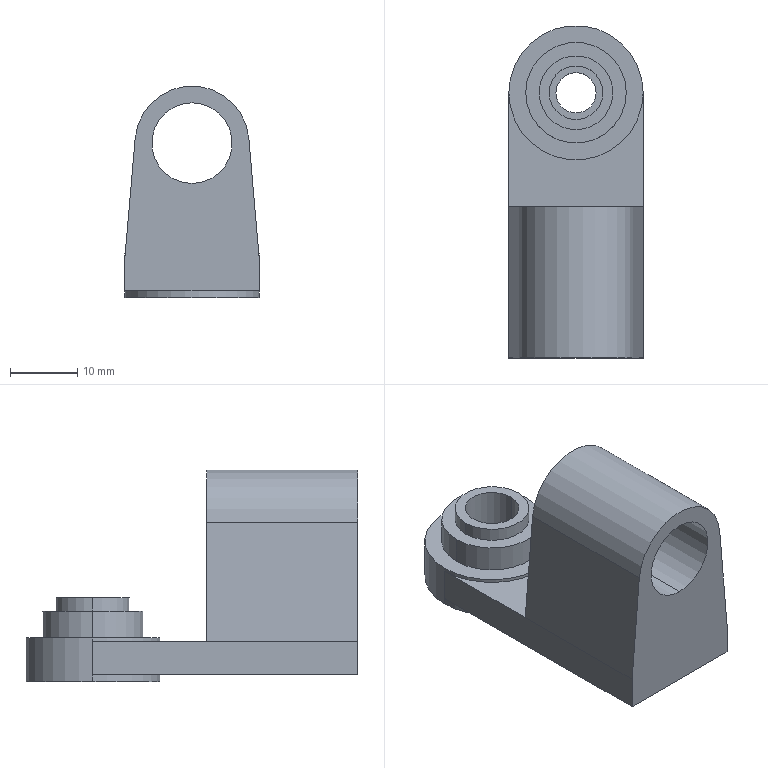Part | STEP file | Polisher L bracket | 1 solid | 27 faces | box 20 x 49.5 x 31.5 mm | volume 12628 mm3 | cylinder 14 | plane 13 | commonest cylinder face diameters 20 x3 6 x2 8 x2 11 x2 12 x2 15 x2